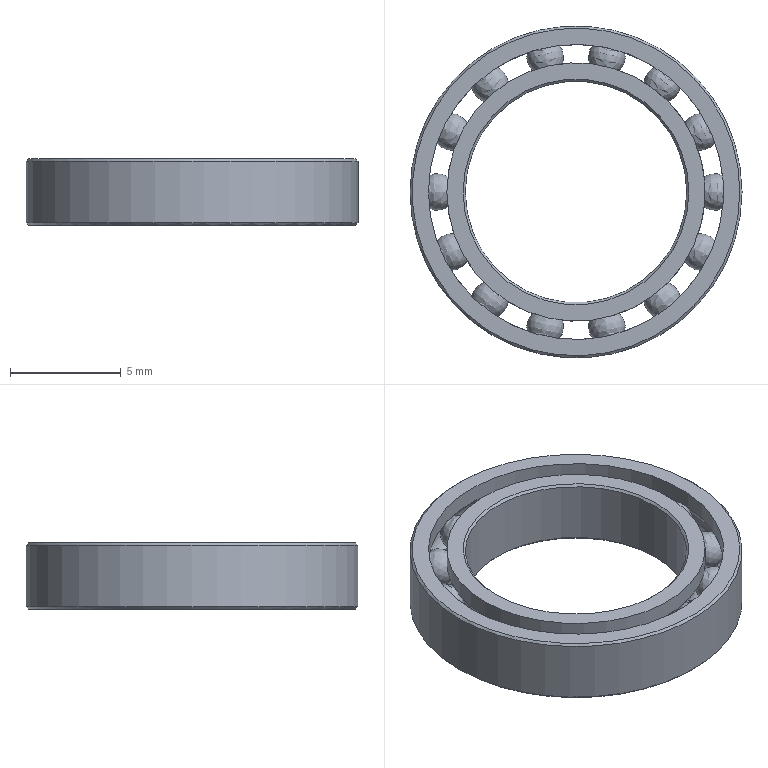Part | NX | features SWP104 18, INSTANCE_SET 13, SKETCH 4, CHAMFER 2, DATUM_CSYS 2, FSET 2, CIRCULAR_PATTERN 1, LINE 1 | 16 solids | 30 faces | box 15 x 15 x 3 mm | volume 196.013 mm3 | sphere 14 | cylinder 6 | plane 4 | cone 4 | torus 2 | commonest cylinder face diameters 11.667 x2 13.333 x2 10 x1 15 x1
STEP:
#1=CARTESIAN_POINT('',(6.667,0.,0.7784));
#2=VERTEX_POINT('',#1);
#3=CARTESIAN_POINT('',(0.,0.,0.7784));
#4=DIRECTION('',(0.,0.,1.));
#5=DIRECTION('',(1.,0.,0.));
#6=AXIS2_PLACEMENT_3D('',#3,#4,#5);
#7=CIRCLE('',#6,6.667);
#8=EDGE_CURVE('',#2,#2,#7,.F.);
#9=ORIENTED_EDGE('',*,*,#8,.F.);
#10=EDGE_LOOP('',(#9));
#11=FACE_BOUND('',#10,.T.);
#12=CARTESIAN_POINT('',(-6.667,0.,0.));
#13=VERTEX_POINT('',#12);
#14=CARTESIAN_POINT('',(0.,0.,0.));
#15=DIRECTION('',(0.,0.,-1.));
#16=DIRECTION('',(-1.,0.,0.));
#17=AXIS2_PLACEMENT_3D('',#14,#15,#16);
#18=CIRCLE('',#17,6.667);
#19=EDGE_CURVE('',#13,#13,#18,.T.);
#20=ORIENTED_EDGE('',*,*,#19,.T.);
#21=EDGE_LOOP('',(#20));
#22=FACE_BOUND('',#21,.T.);
#23=CARTESIAN_POINT('',(0.,0.,0.));
#24=DIRECTION('',(0.,0.,-1.));
#25=DIRECTION('',(-1.,0.,0.));
#26=AXIS2_PLACEMENT_3D('',#23,#24,#25);
#27=CYLINDRICAL_SURFACE('',#26,6.667);
#28=ADVANCED_FACE('',(#11,#22),#27,.F.);
#29=CARTESIAN_POINT('',(-7.5,0.,0.1));
#30=VERTEX_POINT('',#29);
#31=CARTESIAN_POINT('',(0.,0.,0.1));
#32=DIRECTION('',(0.,0.,-1.));
#33=DIRECTION('',(-1.,0.,0.));
#34=AXIS2_PLACEMENT_3D('',#31,#32,#33);
#35=CIRCLE('',#34,7.5);
#36=EDGE_CURVE('',#30,#30,#35,.F.);
#37=ORIENTED_EDGE('',*,*,#36,.T.);
#38=EDGE_LOOP('',(#37));
#39=FACE_BOUND('',#38,.T.);
#40=CARTESIAN_POINT('',(7.5,0.,2.9));
#41=VERTEX_POINT('',#40);
#42=CARTESIAN_POINT('',(0.,0.,2.9));
#43=DIRECTION('',(0.,0.,1.));
#44=DIRECTION('',(1.,0.,0.));
#45=AXIS2_PLACEMENT_3D('',#42,#43,#44);
#46=CIRCLE('',#45,7.5);
#47=EDGE_CURVE('',#41,#41,#46,.F.);
#48=ORIENTED_EDGE('',*,*,#47,.T.);
#49=EDGE_LOOP('',(#48));
#50=FACE_BOUND('',#49,.T.);
#51=CARTESIAN_POINT('',(0.,0.,0.));
#52=DIRECTION('',(0.,0.,-1.));
#53=DIRECTION('',(-1.,0.,0.));
#54=AXIS2_PLACEMENT_3D('',#51,#52,#53);
#55=CYLINDRICAL_SURFACE('',#54,7.5);
#56=ADVANCED_FACE('',(#39,#50),#55,.T.);
#57=CARTESIAN_POINT('',(7.4,0.,3.));
#58=VERTEX_POINT('',#57);
#59=CARTESIAN_POINT('',(0.,0.,3.));
#60=DIRECTION('',(0.,0.,1.));
#61=DIRECTION('',(1.,0.,0.));
#62=AXIS2_PLACEMENT_3D('',#59,#60,#61);
#63=CIRCLE('',#62,7.4);
#64=EDGE_CURVE('',#58,#58,#63,.T.);
#65=ORIENTED_EDGE('',*,*,#64,.T.);
#66=EDGE_LOOP('',(#65));
#67=FACE_BOUND('',#66,.T.);
#68=CARTESIAN_POINT('',(-6.667,0.,3.));
#69=VERTEX_POINT('',#68);
#70=CARTESIAN_POINT('',(0.,0.,3.));
#71=DIRECTION('',(0.,0.,-1.));
#72=DIRECTION('',(-1.,0.,0.));
#73=AXIS2_PLACEMENT_3D('',#70,#71,#72);
#74=CIRCLE('',#73,6.667);
#75=EDGE_CURVE('',#69,#69,#74,.T.);
#76=ORIENTED_EDGE('',*,*,#75,.T.);
#77=EDGE_LOOP('',(#76));
#78=FACE_BOUND('',#77,.T.);
#79=CARTESIAN_POINT('',(7.5,0.,3.));
#80=DIRECTION('',(0.,0.,1.));
#81=DIRECTION('',(1.,0.,0.));
#82=AXIS2_PLACEMENT_3D('',#79,#80,#81);
#83=PLANE('',#82);
#84=ADVANCED_FACE('',(#67,#78),#83,.T.);
#85=CARTESIAN_POINT('',(-6.667,0.,2.222));
#86=VERTEX_POINT('',#85);
#87=CARTESIAN_POINT('',(0.,0.,2.222));
#88=DIRECTION('',(0.,0.,-1.));
#89=DIRECTION('',(-1.,0.,0.));
#90=AXIS2_PLACEMENT_3D('',#87,#88,#89);
#91=CIRCLE('',#90,6.667);
#92=EDGE_CURVE('',#86,#86,#91,.F.);
#93=ORIENTED_EDGE('',*,*,#92,.F.);
#94=EDGE_LOOP('',(#93));
#95=FACE_BOUND('',#94,.T.);
#96=ORIENTED_EDGE('',*,*,#75,.F.);
#97=EDGE_LOOP('',(#96));
#98=FACE_BOUND('',#97,.T.);
#99=CARTESIAN_POINT('',(0.,0.,0.));
#100=DIRECTION('',(0.,0.,-1.));
#101=DIRECTION('',(-1.,0.,0.));
#102=AXIS2_PLACEMENT_3D('',#99,#100,#101);
#103=CYLINDRICAL_SURFACE('',#102,6.667);
#104=ADVANCED_FACE('',(#95,#98),#103,.F.);
#105=CARTESIAN_POINT('',(-7.4,0.,0.));
#106=VERTEX_POINT('',#105);
#107=CARTESIAN_POINT('',(0.,0.,0.));
#108=DIRECTION('',(0.,0.,-1.));
#109=DIRECTION('',(-1.,0.,0.));
#110=AXIS2_PLACEMENT_3D('',#107,#108,#109);
#111=CIRCLE('',#110,7.4);
#112=EDGE_CURVE('',#106,#106,#111,.T.);
#113=ORIENTED_EDGE('',*,*,#112,.T.);
#114=EDGE_LOOP('',(#113));
#115=FACE_BOUND('',#114,.T.);
#116=ORIENTED_EDGE('',*,*,#19,.F.);
#117=EDGE_LOOP('',(#116));
#118=FACE_BOUND('',#117,.T.);
#119=CARTESIAN_POINT('',(6.667,0.,0.));
#120=DIRECTION('',(0.,0.,-1.));
#121=DIRECTION('',(-1.,0.,0.));
#122=AXIS2_PLACEMENT_3D('',#119,#120,#121);
#123=PLANE('',#122);
#124=ADVANCED_FACE('',(#115,#118),#123,.T.);
#125=ORIENTED_EDGE('',*,*,#8,.T.);
#126=EDGE_LOOP('',(#125));
#127=FACE_BOUND('',#126,.T.);
#128=ORIENTED_EDGE('',*,*,#92,.T.);
#129=EDGE_LOOP('',(#128));
#130=FACE_BOUND('',#129,.T.);
#131=CARTESIAN_POINT('',(0.,0.,1.5));
#132=DIRECTION('',(0.,0.,-1.));
#133=DIRECTION('',(-1.,0.,0.));
#134=AXIS2_PLACEMENT_3D('',#131,#132,#133);
#135=TOROIDAL_SURFACE('',#134,6.25,0.8332);
#136=ADVANCED_FACE('',(#127,#130),#135,.F.);
#137=ORIENTED_EDGE('',*,*,#36,.F.);
#138=EDGE_LOOP('',(#137));
#139=FACE_BOUND('',#138,.T.);
#140=ORIENTED_EDGE('',*,*,#112,.F.);
#141=EDGE_LOOP('',(#140));
#142=FACE_BOUND('',#141,.T.);
#143=CARTESIAN_POINT('',(0.,0.,0.));
#144=DIRECTION('',(0.,0.,1.));
#145=DIRECTION('',(1.,0.,0.));
#146=AXIS2_PLACEMENT_3D('',#143,#144,#145);
#147=CONICAL_SURFACE('',#146,7.4,0.7854);
#148=ADVANCED_FACE('',(#139,#142),#147,.T.);
#149=ORIENTED_EDGE('',*,*,#64,.F.);
#150=EDGE_LOOP('',(#149));
#151=FACE_BOUND('',#150,.T.);
#152=ORIENTED_EDGE('',*,*,#47,.F.);
#153=EDGE_LOOP('',(#152));
#154=FACE_BOUND('',#153,.T.);
#155=CARTESIAN_POINT('',(0.,0.,2.9));
#156=DIRECTION('',(0.,0.,-1.));
#157=DIRECTION('',(-1.,0.,0.));
#158=AXIS2_PLACEMENT_3D('',#155,#156,#157);
#159=CONICAL_SURFACE('',#158,7.5,0.7854);
#160=ADVANCED_FACE('',(#151,#154),#159,.T.);
#161=CLOSED_SHELL('',(#28,#56,#84,#104,#124,#136,#148,#160));
#162=MANIFOLD_SOLID_BREP('',#161);
#163=CARTESIAN_POINT('',(5.833,0.,0.7784));
#164=VERTEX_POINT('',#163);
#165=CARTESIAN_POINT('',(0.,0.,0.7784));
#166=DIRECTION('',(0.,0.,1.));
#167=DIRECTION('',(1.,0.,0.));
#168=AXIS2_PLACEMENT_3D('',#165,#166,#167);
#169=CIRCLE('',#168,5.833);
#170=EDGE_CURVE('',#164,#164,#169,.T.);
#171=ORIENTED_EDGE('',*,*,#170,.F.);
#172=EDGE_LOOP('',(#171));
#173=FACE_BOUND('',#172,.T.);
#174=CARTESIAN_POINT('',(-5.833,0.,0.));
#175=VERTEX_POINT('',#174);
#176=CARTESIAN_POINT('',(0.,0.,0.));
#177=DIRECTION('',(0.,0.,-1.));
#178=DIRECTION('',(-1.,0.,0.));
#179=AXIS2_PLACEMENT_3D('',#176,#177,#178);
#180=CIRCLE('',#179,5.833);
#181=EDGE_CURVE('',#175,#175,#180,.T.);
#182=ORIENTED_EDGE('',*,*,#181,.F.);
#183=EDGE_LOOP('',(#182));
#184=FACE_BOUND('',#183,.T.);
#185=CARTESIAN_POINT('',(0.,0.,0.));
#186=DIRECTION('',(0.,0.,-1.));
#187=DIRECTION('',(-1.,0.,0.));
#188=AXIS2_PLACEMENT_3D('',#185,#186,#187);
#189=CYLINDRICAL_SURFACE('',#188,5.833);
#190=ADVANCED_FACE('',(#173,#184),#189,.T.);
#191=CARTESIAN_POINT('',(-5.,0.,0.1));
#192=VERTEX_POINT('',#191);
#193=CARTESIAN_POINT('',(0.,0.,0.1));
#194=DIRECTION('',(0.,0.,-1.));
#195=DIRECTION('',(-1.,0.,0.));
#196=AXIS2_PLACEMENT_3D('',#193,#194,#195);
#197=CIRCLE('',#196,5.);
#198=EDGE_CURVE('',#192,#192,#197,.T.);
#199=ORIENTED_EDGE('',*,*,#198,.T.);
#200=EDGE_LOOP('',(#199));
#201=FACE_BOUND('',#200,.T.);
#202=CARTESIAN_POINT('',(5.,0.,2.9));
#203=VERTEX_POINT('',#202);
#204=CARTESIAN_POINT('',(0.,0.,2.9));
#205=DIRECTION('',(0.,0.,1.));
#206=DIRECTION('',(1.,0.,0.));
#207=AXIS2_PLACEMENT_3D('',#204,#205,#206);
#208=CIRCLE('',#207,5.);
#209=EDGE_CURVE('',#203,#203,#208,.T.);
#210=ORIENTED_EDGE('',*,*,#209,.T.);
#211=EDGE_LOOP('',(#210));
#212=FACE_BOUND('',#211,.T.);
#213=CARTESIAN_POINT('',(0.,0.,0.));
#214=DIRECTION('',(0.,0.,-1.));
#215=DIRECTION('',(-1.,0.,0.));
#216=AXIS2_PLACEMENT_3D('',#213,#214,#215);
#217=CYLINDRICAL_SURFACE('',#216,5.);
#218=ADVANCED_FACE('',(#201,#212),#217,.F.);
#219=CARTESIAN_POINT('',(-5.1,0.,0.));
#220=VERTEX_POINT('',#219);
#221=CARTESIAN_POINT('',(0.,0.,0.));
#222=DIRECTION('',(0.,0.,-1.));
#223=DIRECTION('',(-1.,0.,0.));
#224=AXIS2_PLACEMENT_3D('',#221,#222,#223);
#225=CIRCLE('',#224,5.1);
#226=EDGE_CURVE('',#220,#220,#225,.F.);
#227=ORIENTED_EDGE('',*,*,#226,.T.);
#228=EDGE_LOOP('',(#227));
#229=FACE_BOUND('',#228,.T.);
#230=ORIENTED_EDGE('',*,*,#181,.T.);
#231=EDGE_LOOP('',(#230));
#232=FACE_BOUND('',#231,.T.);
#233=CARTESIAN_POINT('',(5.,0.,0.));
#234=DIRECTION('',(0.,0.,-1.));
#235=DIRECTION('',(-1.,0.,0.));
#236=AXIS2_PLACEMENT_3D('',#233,#234,#235);
#237=PLANE('',#236);
#238=ADVANCED_FACE('',(#229,#232),#237,.T.);
#239=CARTESIAN_POINT('',(-5.833,0.,2.222));
#240=VERTEX_POINT('',#239);
#241=CARTESIAN_POINT('',(0.,0.,2.222));
#242=DIRECTION('',(0.,0.,-1.));
#243=DIRECTION('',(-1.,0.,0.));
#244=AXIS2_PLACEMENT_3D('',#241,#242,#243);
#245=CIRCLE('',#244,5.833);
#246=EDGE_CURVE('',#240,#240,#245,.T.);
#247=ORIENTED_EDGE('',*,*,#246,.F.);
#248=EDGE_LOOP('',(#247));
#249=FACE_BOUND('',#248,.T.);
#250=CARTESIAN_POINT('',(-5.833,0.,3.));
#251=VERTEX_POINT('',#250);
#252=CARTESIAN_POINT('',(0.,0.,3.));
#253=DIRECTION('',(0.,0.,-1.));
#254=DIRECTION('',(-1.,0.,0.));
#255=AXIS2_PLACEMENT_3D('',#252,#253,#254);
#256=CIRCLE('',#255,5.833);
#257=EDGE_CURVE('',#251,#251,#256,.T.);
#258=ORIENTED_EDGE('',*,*,#257,.T.);
#259=EDGE_LOOP('',(#258));
#260=FACE_BOUND('',#259,.T.);
#261=CARTESIAN_POINT('',(0.,0.,0.));
#262=DIRECTION('',(0.,0.,-1.));
#263=DIRECTION('',(-1.,0.,0.));
#264=AXIS2_PLACEMENT_3D('',#261,#262,#263);
#265=CYLINDRICAL_SURFACE('',#264,5.833);
#266=ADVANCED_FACE('',(#249,#260),#265,.T.);
#267=CARTESIAN_POINT('',(5.1,0.,3.));
#268=VERTEX_POINT('',#267);
#269=CARTESIAN_POINT('',(0.,0.,3.));
#270=DIRECTION('',(0.,0.,1.));
#271=DIRECTION('',(1.,0.,0.));
#272=AXIS2_PLACEMENT_3D('',#269,#270,#271);
#273=CIRCLE('',#272,5.1);
#274=EDGE_CURVE('',#268,#268,#273,.F.);
#275=ORIENTED_EDGE('',*,*,#274,.T.);
#276=EDGE_LOOP('',(#275));
#277=FACE_BOUND('',#276,.T.);
#278=ORIENTED_EDGE('',*,*,#257,.F.);
#279=EDGE_LOOP('',(#278));
#280=FACE_BOUND('',#279,.T.);
#281=CARTESIAN_POINT('',(5.833,0.,3.));
#282=DIRECTION('',(0.,0.,1.));
#283=DIRECTION('',(1.,0.,0.));
#284=AXIS2_PLACEMENT_3D('',#281,#282,#283);
#285=PLANE('',#284);
#286=ADVANCED_FACE('',(#277,#280),#285,.T.);
#287=ORIENTED_EDGE('',*,*,#170,.T.);
#288=EDGE_LOOP('',(#287));
#289=FACE_BOUND('',#288,.T.);
#290=ORIENTED_EDGE('',*,*,#246,.T.);
#291=EDGE_LOOP('',(#290));
#292=FACE_BOUND('',#291,.T.);
#293=CARTESIAN_POINT('',(0.,0.,1.5));
#294=DIRECTION('',(0.,0.,-1.));
#295=DIRECTION('',(-1.,0.,0.));
#296=AXIS2_PLACEMENT_3D('',#293,#294,#295);
#297=TOROIDAL_SURFACE('',#296,6.25,0.8332);
#298=ADVANCED_FACE('',(#289,#292),#297,.F.);
#299=ORIENTED_EDGE('',*,*,#226,.F.);
#300=EDGE_LOOP('',(#299));
#301=FACE_BOUND('',#300,.T.);
#302=ORIENTED_EDGE('',*,*,#198,.F.);
#303=EDGE_LOOP('',(#302));
#304=FACE_BOUND('',#303,.T.);
#305=CARTESIAN_POINT('',(0.,0.,0.1));
#306=DIRECTION('',(0.,0.,-1.));
#307=DIRECTION('',(-1.,0.,0.));
#308=AXIS2_PLACEMENT_3D('',#305,#306,#307);
#309=CONICAL_SURFACE('',#308,5.,0.7854);
#310=ADVANCED_FACE('',(#301,#304),#309,.F.);
#311=ORIENTED_EDGE('',*,*,#209,.F.);
#312=EDGE_LOOP('',(#311));
#313=FACE_BOUND('',#312,.T.);
#314=ORIENTED_EDGE('',*,*,#274,.F.);
#315=EDGE_LOOP('',(#314));
#316=FACE_BOUND('',#315,.T.);
#317=CARTESIAN_POINT('',(0.,0.,3.));
#318=DIRECTION('',(0.,0.,1.));
#319=DIRECTION('',(1.,0.,0.));
#320=AXIS2_PLACEMENT_3D('',#317,#318,#319);
#321=CONICAL_SURFACE('',#320,5.1,0.7854);
#322=ADVANCED_FACE('',(#313,#316),#321,.F.);
#323=CLOSED_SHELL('',(#190,#218,#238,#266,#286,#298,#310,#322));
#324=MANIFOLD_SOLID_BREP('',#323);
#325=CARTESIAN_POINT('',(5.417,0.,1.5));
#326=VERTEX_POINT('',#325);
#327=VERTEX_LOOP('',#326);
#328=FACE_BOUND('',#327,.T.);
#329=CARTESIAN_POINT('',(6.25,0.,1.5));
#330=DIRECTION('',(1.,0.,0.));
#331=DIRECTION('',(0.,0.,1.));
#332=AXIS2_PLACEMENT_3D('',#329,#330,#331);
#333=SPHERICAL_SURFACE('',#332,0.8332);
#334=ADVANCED_FACE('',(#328),#333,.T.);
#335=CLOSED_SHELL('',(#334));
#336=MANIFOLD_SOLID_BREP('',#335);
#337=CARTESIAN_POINT('',(4.88,2.35,1.5));
#338=VERTEX_POINT('',#337);
#339=VERTEX_LOOP('',#338);
#340=FACE_BOUND('',#339,.T.);
#341=CARTESIAN_POINT('',(5.631,2.712,1.5));
#342=DIRECTION('',(0.901,0.4339,0.));
#343=DIRECTION('',(0.,0.,1.));
#344=AXIS2_PLACEMENT_3D('',#341,#342,#343);
#345=SPHERICAL_SURFACE('',#344,0.8332);
#346=ADVANCED_FACE('',(#340),#345,.T.);
#347=CLOSED_SHELL('',(#346));
#348=MANIFOLD_SOLID_BREP('',#347);
#349=CARTESIAN_POINT('',(3.377,4.235,1.5));
#350=VERTEX_POINT('',#349);
#351=VERTEX_LOOP('',#350);
#352=FACE_BOUND('',#351,.T.);
#353=CARTESIAN_POINT('',(3.897,4.886,1.5));
#354=DIRECTION('',(0.6235,0.7818,0.));
#355=DIRECTION('',(0.,0.,1.));
#356=AXIS2_PLACEMENT_3D('',#353,#354,#355);
#357=SPHERICAL_SURFACE('',#356,0.8332);
#358=ADVANCED_FACE('',(#352),#357,.T.);
#359=CLOSED_SHELL('',(#358));
#360=MANIFOLD_SOLID_BREP('',#359);
#361=CARTESIAN_POINT('',(1.205,5.281,1.5));
#362=VERTEX_POINT('',#361);
#363=VERTEX_LOOP('',#362);
#364=FACE_BOUND('',#363,.T.);
#365=CARTESIAN_POINT('',(1.391,6.093,1.5));
#366=DIRECTION('',(0.2225,0.9749,0.));
#367=DIRECTION('',(0.,0.,1.));
#368=AXIS2_PLACEMENT_3D('',#365,#366,#367);
#369=SPHERICAL_SURFACE('',#368,0.8332);
#370=ADVANCED_FACE('',(#364),#369,.T.);
#371=CLOSED_SHELL('',(#370));
#372=MANIFOLD_SOLID_BREP('',#371);
#373=CARTESIAN_POINT('',(-1.205,5.281,1.5));
#374=VERTEX_POINT('',#373);
#375=VERTEX_LOOP('',#374);
#376=FACE_BOUND('',#375,.T.);
#377=CARTESIAN_POINT('',(-1.391,6.093,1.5));
#378=DIRECTION('',(-0.2225,0.9749,0.));
#379=DIRECTION('',(0.,0.,1.));
#380=AXIS2_PLACEMENT_3D('',#377,#378,#379);
#381=SPHERICAL_SURFACE('',#380,0.8332);
#382=ADVANCED_FACE('',(#376),#381,.T.);
#383=CLOSED_SHELL('',(#382));
#384=MANIFOLD_SOLID_BREP('',#383);
#385=CARTESIAN_POINT('',(-3.377,4.235,1.5));
#386=VERTEX_POINT('',#385);
#387=VERTEX_LOOP('',#386);
#388=FACE_BOUND('',#387,.T.);
#389=CARTESIAN_POINT('',(-3.897,4.886,1.5));
#390=DIRECTION('',(-0.6235,0.7818,0.));
#391=DIRECTION('',(0.,0.,1.));
#392=AXIS2_PLACEMENT_3D('',#389,#390,#391);
#393=SPHERICAL_SURFACE('',#392,0.8332);
#394=ADVANCED_FACE('',(#388),#393,.T.);
#395=CLOSED_SHELL('',(#394));
#396=MANIFOLD_SOLID_BREP('',#395);
#397=CARTESIAN_POINT('',(-4.88,2.35,1.5));
#398=VERTEX_POINT('',#397);
#399=VERTEX_LOOP('',#398);
#400=FACE_BOUND('',#399,.T.);
#401=CARTESIAN_POINT('',(-5.631,2.712,1.5));
#402=DIRECTION('',(-0.901,0.4339,0.));
#403=DIRECTION('',(0.,0.,1.));
#404=AXIS2_PLACEMENT_3D('',#401,#402,#403);
#405=SPHERICAL_SURFACE('',#404,0.8332);
#406=ADVANCED_FACE('',(#400),#405,.T.);
#407=CLOSED_SHELL('',(#406));
#408=MANIFOLD_SOLID_BREP('',#407);
#409=CARTESIAN_POINT('',(-5.417,0.,1.5));
#410=VERTEX_POINT('',#409);
#411=VERTEX_LOOP('',#410);
#412=FACE_BOUND('',#411,.T.);
#413=CARTESIAN_POINT('',(-6.25,0.,1.5));
#414=DIRECTION('',(-1.,0.,0.));
#415=DIRECTION('',(0.,0.,1.));
#416=AXIS2_PLACEMENT_3D('',#413,#414,#415);
#417=SPHERICAL_SURFACE('',#416,0.8332);
#418=ADVANCED_FACE('',(#412),#417,.T.);
#419=CLOSED_SHELL('',(#418));
#420=MANIFOLD_SOLID_BREP('',#419);
#421=CARTESIAN_POINT('',(-4.88,-2.35,1.5));
#422=VERTEX_POINT('',#421);
#423=VERTEX_LOOP('',#422);
#424=FACE_BOUND('',#423,.T.);
#425=CARTESIAN_POINT('',(-5.631,-2.712,1.5));
#426=DIRECTION('',(-0.901,-0.4339,0.));
#427=DIRECTION('',(0.,0.,1.));
#428=AXIS2_PLACEMENT_3D('',#425,#426,#427);
#429=SPHERICAL_SURFACE('',#428,0.8332);
#430=ADVANCED_FACE('',(#424),#429,.T.);
#431=CLOSED_SHELL('',(#430));
#432=MANIFOLD_SOLID_BREP('',#431);
#433=CARTESIAN_POINT('',(-3.377,-4.235,1.5));
#434=VERTEX_POINT('',#433);
#435=VERTEX_LOOP('',#434);
#436=FACE_BOUND('',#435,.T.);
#437=CARTESIAN_POINT('',(-3.897,-4.886,1.5));
#438=DIRECTION('',(-0.6235,-0.7818,0.));
#439=DIRECTION('',(0.,0.,1.));
#440=AXIS2_PLACEMENT_3D('',#437,#438,#439);
#441=SPHERICAL_SURFACE('',#440,0.8332);
#442=ADVANCED_FACE('',(#436),#441,.T.);
#443=CLOSED_SHELL('',(#442));
#444=MANIFOLD_SOLID_BREP('',#443);
#445=CARTESIAN_POINT('',(-1.205,-5.281,1.5));
#446=VERTEX_POINT('',#445);
#447=VERTEX_LOOP('',#446);
#448=FACE_BOUND('',#447,.T.);
#449=CARTESIAN_POINT('',(-1.391,-6.093,1.5));
#450=DIRECTION('',(-0.2225,-0.9749,0.));
#451=DIRECTION('',(0.,0.,1.));
#452=AXIS2_PLACEMENT_3D('',#449,#450,#451);
#453=SPHERICAL_SURFACE('',#452,0.8332);
#454=ADVANCED_FACE('',(#448),#453,.T.);
#455=CLOSED_SHELL('',(#454));
#456=MANIFOLD_SOLID_BREP('',#455);
#457=CARTESIAN_POINT('',(1.205,-5.281,1.5));
#458=VERTEX_POINT('',#457);
#459=VERTEX_LOOP('',#458);
#460=FACE_BOUND('',#459,.T.);
#461=CARTESIAN_POINT('',(1.391,-6.093,1.5));
#462=DIRECTION('',(0.2225,-0.9749,0.));
#463=DIRECTION('',(0.,0.,1.));
#464=AXIS2_PLACEMENT_3D('',#461,#462,#463);
#465=SPHERICAL_SURFACE('',#464,0.8332);
#466=ADVANCED_FACE('',(#460),#465,.T.);
#467=CLOSED_SHELL('',(#466));
#468=MANIFOLD_SOLID_BREP('',#467);
#469=CARTESIAN_POINT('',(3.377,-4.235,1.5));
#470=VERTEX_POINT('',#469);
#471=VERTEX_LOOP('',#470);
#472=FACE_BOUND('',#471,.T.);
#473=CARTESIAN_POINT('',(3.897,-4.886,1.5));
#474=DIRECTION('',(0.6235,-0.7818,0.));
#475=DIRECTION('',(0.,0.,1.));
#476=AXIS2_PLACEMENT_3D('',#473,#474,#475);
#477=SPHERICAL_SURFACE('',#476,0.8332);
#478=ADVANCED_FACE('',(#472),#477,.T.);
#479=CLOSED_SHELL('',(#478));
#480=MANIFOLD_SOLID_BREP('',#479);
#481=CARTESIAN_POINT('',(4.88,-2.35,1.5));
#482=VERTEX_POINT('',#481);
#483=VERTEX_LOOP('',#482);
#484=FACE_BOUND('',#483,.T.);
#485=CARTESIAN_POINT('',(5.631,-2.712,1.5));
#486=DIRECTION('',(0.901,-0.4339,0.));
#487=DIRECTION('',(0.,0.,1.));
#488=AXIS2_PLACEMENT_3D('',#485,#486,#487);
#489=SPHERICAL_SURFACE('',#488,0.8332);
#490=ADVANCED_FACE('',(#484),#489,.T.);
#491=CLOSED_SHELL('',(#490));
#492=MANIFOLD_SOLID_BREP('',#491);
#493=(LENGTH_UNIT()NAMED_UNIT(*)SI_UNIT(.MILLI.,.METRE.));
#494=UNCERTAINTY_MEASURE_WITH_UNIT(LENGTH_MEASURE(0.00001),#493,'','');
#495=(NAMED_UNIT(*)PLANE_ANGLE_UNIT()SI_UNIT($,.RADIAN.));
#496=(NAMED_UNIT(*)SI_UNIT($,.STERADIAN.)SOLID_ANGLE_UNIT());
#497=(GEOMETRIC_REPRESENTATION_CONTEXT(3)GLOBAL_UNCERTAINTY_ASSIGNED_CONTEXT((#494))GLOBAL_UNIT_ASSIGNED_CONTEXT((#493,#495,#496))REPRESENTATION_CONTEXT('',''));
#498=ADVANCED_BREP_SHAPE_REPRESENTATION('',(#162,#324,#336,#348,#360,#372,#384,#396,#408,#420,#432,#444,#456,#468,#480,#492),#497);